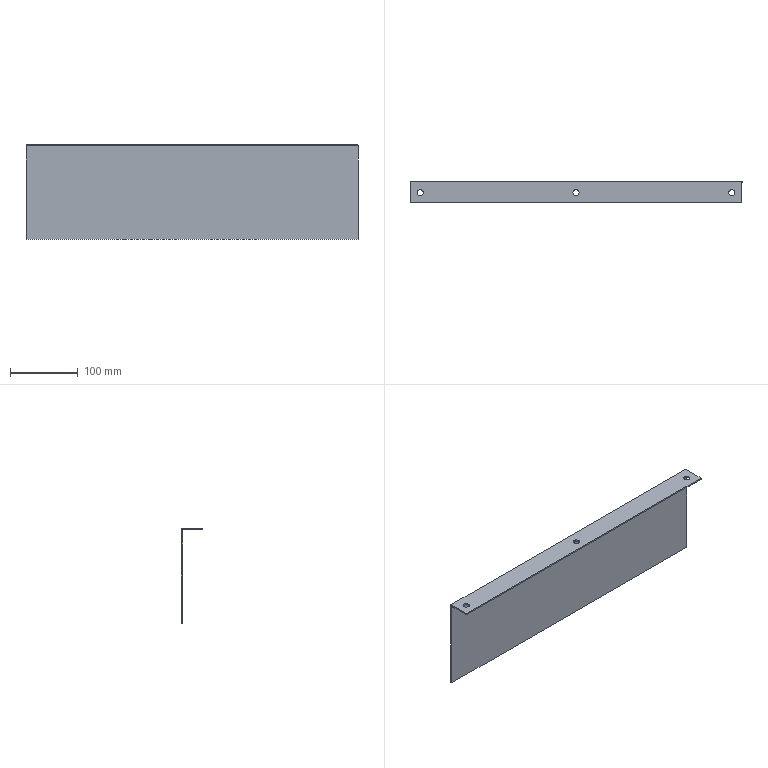Part | STEP file | lll_id2766_x_t | 1 solid | 11 faces | box 490 x 32 x 140 mm | volume 166218 mm3 | plane 8 | cylinder 3 | commonest cylinder face diameters 9 x3
STEP:
#1=CARTESIAN_POINT('',(949.935,-441.,2.5));
#2=VERTEX_POINT('',#1);
#3=CARTESIAN_POINT('',(949.935,-439.,2.5));
#4=VERTEX_POINT('',#3);
#5=CARTESIAN_POINT('',(949.935,-441.,2.5));
#6=DIRECTION('',(0.,1.,0.));
#7=VECTOR('',#6,1.);
#8=LINE('',#5,#7);
#9=EDGE_CURVE('',#2,#4,#8,.T.);
#10=ORIENTED_EDGE('',*,*,#9,.T.);
#11=CARTESIAN_POINT('',(1439.935,-439.,2.5));
#12=VERTEX_POINT('',#11);
#13=CARTESIAN_POINT('',(949.935,-439.,2.5));
#14=DIRECTION('',(1.,0.,0.));
#15=VECTOR('',#14,1.);
#16=LINE('',#13,#15);
#17=EDGE_CURVE('',#4,#12,#16,.T.);
#18=ORIENTED_EDGE('',*,*,#17,.T.);
#19=CARTESIAN_POINT('',(1439.935,-441.,2.5));
#20=VERTEX_POINT('',#19);
#21=CARTESIAN_POINT('',(1439.935,45.,2.5));
#22=DIRECTION('',(0.,1.,0.));
#23=VECTOR('',#22,1.);
#24=LINE('',#21,#23);
#25=EDGE_CURVE('',#20,#12,#24,.T.);
#26=ORIENTED_EDGE('',*,*,#25,.F.);
#27=CARTESIAN_POINT('',(949.935,-441.,2.5));
#28=DIRECTION('',(1.,0.,0.));
#29=VECTOR('',#28,1.);
#30=LINE('',#27,#29);
#31=EDGE_CURVE('',#2,#20,#30,.T.);
#32=ORIENTED_EDGE('',*,*,#31,.F.);
#33=EDGE_LOOP('',(#10,#18,#26,#32));
#34=FACE_OUTER_BOUND('',#33,.T.);
#35=CARTESIAN_POINT('',(2142.435,45.,2.5));
#36=DIRECTION('',(0.,0.,-1.));
#37=DIRECTION('',(-1.,0.,0.));
#38=AXIS2_PLACEMENT_3D('',#35,#36,#37);
#39=PLANE('',#38);
#40=ADVANCED_FACE('',(#34),#39,.T.);
#41=CARTESIAN_POINT('',(1439.935,-441.,140.5));
#42=VERTEX_POINT('',#41);
#43=CARTESIAN_POINT('',(949.935,-441.,140.5));
#44=VERTEX_POINT('',#43);
#45=CARTESIAN_POINT('',(949.935,-441.,140.5));
#46=DIRECTION('',(-1.,0.,0.));
#47=VECTOR('',#46,1.);
#48=LINE('',#45,#47);
#49=EDGE_CURVE('',#42,#44,#48,.T.);
#50=ORIENTED_EDGE('',*,*,#49,.T.);
#51=CARTESIAN_POINT('',(949.935,-441.,142.5));
#52=DIRECTION('',(0.,0.,-1.));
#53=VECTOR('',#52,1.);
#54=LINE('',#51,#53);
#55=EDGE_CURVE('',#44,#2,#54,.T.);
#56=ORIENTED_EDGE('',*,*,#55,.T.);
#57=ORIENTED_EDGE('',*,*,#31,.T.);
#58=CARTESIAN_POINT('',(1439.935,-441.,-78.5));
#59=DIRECTION('',(0.,0.,1.));
#60=VECTOR('',#59,1.);
#61=LINE('',#58,#60);
#62=EDGE_CURVE('',#20,#42,#61,.T.);
#63=ORIENTED_EDGE('',*,*,#62,.T.);
#64=EDGE_LOOP('',(#50,#56,#57,#63));
#65=FACE_OUTER_BOUND('',#64,.T.);
#66=CARTESIAN_POINT('',(949.935,-441.,-78.5));
#67=DIRECTION('',(0.,1.,0.));
#68=DIRECTION('',(0.,0.,-1.));
#69=AXIS2_PLACEMENT_3D('',#66,#67,#68);
#70=PLANE('',#69);
#71=ADVANCED_FACE('',(#65),#70,.F.);
#72=CARTESIAN_POINT('',(949.935,-439.,142.5));
#73=VERTEX_POINT('',#72);
#74=CARTESIAN_POINT('',(949.935,-439.,-78.5));
#75=DIRECTION('',(0.,0.,-1.));
#76=VECTOR('',#75,1.);
#77=LINE('',#74,#76);
#78=EDGE_CURVE('',#73,#4,#77,.T.);
#79=ORIENTED_EDGE('',*,*,#78,.F.);
#80=CARTESIAN_POINT('',(1439.935,-439.,142.5));
#81=VERTEX_POINT('',#80);
#82=CARTESIAN_POINT('',(949.935,-439.,142.5));
#83=DIRECTION('',(-1.,0.,0.));
#84=VECTOR('',#83,1.);
#85=LINE('',#82,#84);
#86=EDGE_CURVE('',#81,#73,#85,.T.);
#87=ORIENTED_EDGE('',*,*,#86,.F.);
#88=CARTESIAN_POINT('',(1439.935,-439.,-78.5));
#89=DIRECTION('',(0.,0.,1.));
#90=VECTOR('',#89,1.);
#91=LINE('',#88,#90);
#92=EDGE_CURVE('',#12,#81,#91,.T.);
#93=ORIENTED_EDGE('',*,*,#92,.F.);
#94=ORIENTED_EDGE('',*,*,#17,.F.);
#95=EDGE_LOOP('',(#79,#87,#93,#94));
#96=FACE_OUTER_BOUND('',#95,.T.);
#97=CARTESIAN_POINT('',(949.935,-439.,-78.5));
#98=DIRECTION('',(0.,1.,0.));
#99=DIRECTION('',(0.,0.,-1.));
#100=AXIS2_PLACEMENT_3D('',#97,#98,#99);
#101=PLANE('',#100);
#102=ADVANCED_FACE('',(#96),#101,.T.);
#103=ORIENTED_EDGE('',*,*,#9,.F.);
#104=ORIENTED_EDGE('',*,*,#55,.F.);
#105=CARTESIAN_POINT('',(949.935,-471.,140.5));
#106=VERTEX_POINT('',#105);
#107=CARTESIAN_POINT('',(949.935,-441.,140.5));
#108=DIRECTION('',(0.,1.,0.));
#109=VECTOR('',#108,1.);
#110=LINE('',#107,#109);
#111=EDGE_CURVE('',#106,#44,#110,.T.);
#112=ORIENTED_EDGE('',*,*,#111,.F.);
#113=CARTESIAN_POINT('',(949.935,-471.,142.5));
#114=VERTEX_POINT('',#113);
#115=CARTESIAN_POINT('',(949.935,-471.,142.5));
#116=DIRECTION('',(0.,0.,-1.));
#117=VECTOR('',#116,1.);
#118=LINE('',#115,#117);
#119=EDGE_CURVE('',#114,#106,#118,.T.);
#120=ORIENTED_EDGE('',*,*,#119,.F.);
#121=CARTESIAN_POINT('',(949.935,-441.,142.5));
#122=DIRECTION('',(0.,1.,0.));
#123=VECTOR('',#122,1.);
#124=LINE('',#121,#123);
#125=EDGE_CURVE('',#114,#73,#124,.T.);
#126=ORIENTED_EDGE('',*,*,#125,.T.);
#127=ORIENTED_EDGE('',*,*,#78,.T.);
#128=EDGE_LOOP('',(#103,#104,#112,#120,#126,#127));
#129=FACE_OUTER_BOUND('',#128,.T.);
#130=CARTESIAN_POINT('',(949.935,-441.,142.5));
#131=DIRECTION('',(-1.,0.,0.));
#132=DIRECTION('',(0.,0.,-1.));
#133=AXIS2_PLACEMENT_3D('',#130,#131,#132);
#134=PLANE('',#133);
#135=ADVANCED_FACE('',(#129),#134,.T.);
#136=ORIENTED_EDGE('',*,*,#119,.T.);
#137=CARTESIAN_POINT('',(1439.935,-471.,140.5));
#138=VERTEX_POINT('',#137);
#139=CARTESIAN_POINT('',(949.935,-471.,140.5));
#140=DIRECTION('',(-1.,0.,0.));
#141=VECTOR('',#140,1.);
#142=LINE('',#139,#141);
#143=EDGE_CURVE('',#138,#106,#142,.T.);
#144=ORIENTED_EDGE('',*,*,#143,.F.);
#145=CARTESIAN_POINT('',(1439.935,-471.,142.5));
#146=VERTEX_POINT('',#145);
#147=CARTESIAN_POINT('',(1439.935,-471.,142.5));
#148=DIRECTION('',(0.,0.,-1.));
#149=VECTOR('',#148,1.);
#150=LINE('',#147,#149);
#151=EDGE_CURVE('',#146,#138,#150,.T.);
#152=ORIENTED_EDGE('',*,*,#151,.F.);
#153=CARTESIAN_POINT('',(949.935,-471.,142.5));
#154=DIRECTION('',(-1.,0.,0.));
#155=VECTOR('',#154,1.);
#156=LINE('',#153,#155);
#157=EDGE_CURVE('',#146,#114,#156,.T.);
#158=ORIENTED_EDGE('',*,*,#157,.T.);
#159=EDGE_LOOP('',(#136,#144,#152,#158));
#160=FACE_OUTER_BOUND('',#159,.T.);
#161=CARTESIAN_POINT('',(949.935,-471.,142.5));
#162=DIRECTION('',(0.,-1.,0.));
#163=DIRECTION('',(1.,0.,0.));
#164=AXIS2_PLACEMENT_3D('',#161,#162,#163);
#165=PLANE('',#164);
#166=ADVANCED_FACE('',(#160),#165,.T.);
#167=CARTESIAN_POINT('',(1439.935,-441.,142.5));
#168=DIRECTION('',(0.,1.,0.));
#169=VECTOR('',#168,1.);
#170=LINE('',#167,#169);
#171=EDGE_CURVE('',#146,#81,#170,.T.);
#172=ORIENTED_EDGE('',*,*,#171,.F.);
#173=ORIENTED_EDGE('',*,*,#151,.T.);
#174=CARTESIAN_POINT('',(1439.935,-441.,140.5));
#175=DIRECTION('',(0.,1.,0.));
#176=VECTOR('',#175,1.);
#177=LINE('',#174,#176);
#178=EDGE_CURVE('',#138,#42,#177,.T.);
#179=ORIENTED_EDGE('',*,*,#178,.T.);
#180=ORIENTED_EDGE('',*,*,#62,.F.);
#181=ORIENTED_EDGE('',*,*,#25,.T.);
#182=ORIENTED_EDGE('',*,*,#92,.T.);
#183=EDGE_LOOP('',(#172,#173,#179,#180,#181,#182));
#184=FACE_OUTER_BOUND('',#183,.T.);
#185=CARTESIAN_POINT('',(1439.935,-441.,-78.5));
#186=DIRECTION('',(-1.,0.,0.));
#187=DIRECTION('',(0.,0.,-1.));
#188=AXIS2_PLACEMENT_3D('',#185,#186,#187);
#189=PLANE('',#188);
#190=ADVANCED_FACE('',(#184),#189,.F.);
#191=CARTESIAN_POINT('',(1420.435,-456.,142.5));
#192=VERTEX_POINT('',#191);
#193=CARTESIAN_POINT('',(1424.935,-456.,142.5));
#194=DIRECTION('',(0.,0.,-1.));
#195=DIRECTION('',(-1.,0.,0.));
#196=AXIS2_PLACEMENT_3D('',#193,#194,#195);
#197=CIRCLE('',#196,4.5);
#198=EDGE_CURVE('',#192,#192,#197,.T.);
#199=ORIENTED_EDGE('',*,*,#198,.F.);
#200=EDGE_LOOP('',(#199));
#201=FACE_BOUND('',#200,.T.);
#202=CARTESIAN_POINT('',(1429.435,-456.,140.5));
#203=VERTEX_POINT('',#202);
#204=CARTESIAN_POINT('',(1424.935,-456.,140.5));
#205=DIRECTION('',(0.,0.,-1.));
#206=DIRECTION('',(1.,0.,0.));
#207=AXIS2_PLACEMENT_3D('',#204,#205,#206);
#208=CIRCLE('',#207,4.5);
#209=EDGE_CURVE('',#203,#203,#208,.T.);
#210=ORIENTED_EDGE('',*,*,#209,.T.);
#211=EDGE_LOOP('',(#210));
#212=FACE_BOUND('',#211,.T.);
#213=CARTESIAN_POINT('',(1424.935,-456.,140.5));
#214=DIRECTION('',(0.,0.,1.));
#215=DIRECTION('',(1.,0.,0.));
#216=AXIS2_PLACEMENT_3D('',#213,#214,#215);
#217=CYLINDRICAL_SURFACE('',#216,4.5);
#218=ADVANCED_FACE('',(#201,#212),#217,.F.);
#219=CARTESIAN_POINT('',(960.435,-456.,142.5));
#220=VERTEX_POINT('',#219);
#221=CARTESIAN_POINT('',(964.935,-456.,142.5));
#222=DIRECTION('',(0.,0.,-1.));
#223=DIRECTION('',(-1.,0.,0.));
#224=AXIS2_PLACEMENT_3D('',#221,#222,#223);
#225=CIRCLE('',#224,4.5);
#226=EDGE_CURVE('',#220,#220,#225,.T.);
#227=ORIENTED_EDGE('',*,*,#226,.F.);
#228=EDGE_LOOP('',(#227));
#229=FACE_BOUND('',#228,.T.);
#230=CARTESIAN_POINT('',(960.435,-456.,140.5));
#231=VERTEX_POINT('',#230);
#232=CARTESIAN_POINT('',(964.935,-456.,140.5));
#233=DIRECTION('',(0.,0.,-1.));
#234=DIRECTION('',(-1.,0.,0.));
#235=AXIS2_PLACEMENT_3D('',#232,#233,#234);
#236=CIRCLE('',#235,4.5);
#237=EDGE_CURVE('',#231,#231,#236,.T.);
#238=ORIENTED_EDGE('',*,*,#237,.T.);
#239=EDGE_LOOP('',(#238));
#240=FACE_BOUND('',#239,.T.);
#241=CARTESIAN_POINT('',(964.935,-456.,140.5));
#242=DIRECTION('',(0.,0.,1.));
#243=DIRECTION('',(-1.,0.,0.));
#244=AXIS2_PLACEMENT_3D('',#241,#242,#243);
#245=CYLINDRICAL_SURFACE('',#244,4.5);
#246=ADVANCED_FACE('',(#229,#240),#245,.F.);
#247=CARTESIAN_POINT('',(1190.435,-456.,142.5));
#248=VERTEX_POINT('',#247);
#249=CARTESIAN_POINT('',(1194.935,-456.,142.5));
#250=DIRECTION('',(0.,0.,-1.));
#251=DIRECTION('',(-1.,0.,0.));
#252=AXIS2_PLACEMENT_3D('',#249,#250,#251);
#253=CIRCLE('',#252,4.5);
#254=EDGE_CURVE('',#248,#248,#253,.T.);
#255=ORIENTED_EDGE('',*,*,#254,.T.);
#256=EDGE_LOOP('',(#255));
#257=FACE_BOUND('',#256,.T.);
#258=ORIENTED_EDGE('',*,*,#226,.T.);
#259=EDGE_LOOP('',(#258));
#260=FACE_BOUND('',#259,.T.);
#261=ORIENTED_EDGE('',*,*,#198,.T.);
#262=EDGE_LOOP('',(#261));
#263=FACE_BOUND('',#262,.T.);
#264=ORIENTED_EDGE('',*,*,#171,.T.);
#265=ORIENTED_EDGE('',*,*,#86,.T.);
#266=ORIENTED_EDGE('',*,*,#125,.F.);
#267=ORIENTED_EDGE('',*,*,#157,.F.);
#268=EDGE_LOOP('',(#264,#265,#266,#267));
#269=FACE_BOUND('',#268,.T.);
#270=CARTESIAN_POINT('',(949.935,-441.,142.5));
#271=DIRECTION('',(0.,0.,-1.));
#272=DIRECTION('',(1.,0.,0.));
#273=AXIS2_PLACEMENT_3D('',#270,#271,#272);
#274=PLANE('',#273);
#275=ADVANCED_FACE('',(#257,#260,#263,#269),#274,.F.);
#276=CARTESIAN_POINT('',(1190.435,-456.,140.5));
#277=VERTEX_POINT('',#276);
#278=CARTESIAN_POINT('',(1194.935,-456.,140.5));
#279=DIRECTION('',(0.,0.,-1.));
#280=DIRECTION('',(-1.,0.,0.));
#281=AXIS2_PLACEMENT_3D('',#278,#279,#280);
#282=CIRCLE('',#281,4.5);
#283=EDGE_CURVE('',#277,#277,#282,.T.);
#284=ORIENTED_EDGE('',*,*,#283,.F.);
#285=EDGE_LOOP('',(#284));
#286=FACE_BOUND('',#285,.T.);
#287=ORIENTED_EDGE('',*,*,#237,.F.);
#288=EDGE_LOOP('',(#287));
#289=FACE_BOUND('',#288,.T.);
#290=ORIENTED_EDGE('',*,*,#209,.F.);
#291=EDGE_LOOP('',(#290));
#292=FACE_BOUND('',#291,.T.);
#293=ORIENTED_EDGE('',*,*,#178,.F.);
#294=ORIENTED_EDGE('',*,*,#143,.T.);
#295=ORIENTED_EDGE('',*,*,#111,.T.);
#296=ORIENTED_EDGE('',*,*,#49,.F.);
#297=EDGE_LOOP('',(#293,#294,#295,#296));
#298=FACE_BOUND('',#297,.T.);
#299=CARTESIAN_POINT('',(949.935,-441.,140.5));
#300=DIRECTION('',(0.,0.,-1.));
#301=DIRECTION('',(1.,0.,0.));
#302=AXIS2_PLACEMENT_3D('',#299,#300,#301);
#303=PLANE('',#302);
#304=ADVANCED_FACE('',(#286,#289,#292,#298),#303,.T.);
#305=ORIENTED_EDGE('',*,*,#254,.F.);
#306=EDGE_LOOP('',(#305));
#307=FACE_BOUND('',#306,.T.);
#308=ORIENTED_EDGE('',*,*,#283,.T.);
#309=EDGE_LOOP('',(#308));
#310=FACE_BOUND('',#309,.T.);
#311=CARTESIAN_POINT('',(1194.935,-456.,140.5));
#312=DIRECTION('',(0.,0.,1.));
#313=DIRECTION('',(1.,0.,0.));
#314=AXIS2_PLACEMENT_3D('',#311,#312,#313);
#315=CYLINDRICAL_SURFACE('',#314,4.5);
#316=ADVANCED_FACE('',(#307,#310),#315,.F.);
#317=CLOSED_SHELL('',(#40,#71,#102,#135,#166,#190,#218,#246,#275,#304,#316));
#318=MANIFOLD_SOLID_BREP('',#317);
#319=(LENGTH_UNIT()NAMED_UNIT(*)SI_UNIT(.MILLI.,.METRE.));
#320=UNCERTAINTY_MEASURE_WITH_UNIT(LENGTH_MEASURE(0.00002),#319,'','');
#321=(NAMED_UNIT(*)PLANE_ANGLE_UNIT()SI_UNIT($,.RADIAN.));
#322=PLANE_ANGLE_MEASURE_WITH_UNIT(PLANE_ANGLE_MEASURE(0.01745),#321);
#323=DIMENSIONAL_EXPONENTS(0.,0.,0.,0.,0.,0.,0.);
#324=(CONVERSION_BASED_UNIT('DEGREE',#322)NAMED_UNIT(#323)PLANE_ANGLE_UNIT());
#325=(NAMED_UNIT(*)SI_UNIT($,.STERADIAN.)SOLID_ANGLE_UNIT());
#326=(GEOMETRIC_REPRESENTATION_CONTEXT(3)GLOBAL_UNCERTAINTY_ASSIGNED_CONTEXT((#320))GLOBAL_UNIT_ASSIGNED_CONTEXT((#319,#324,#325))REPRESENTATION_CONTEXT('',''));
#327=ADVANCED_BREP_SHAPE_REPRESENTATION('',(#318),#326);